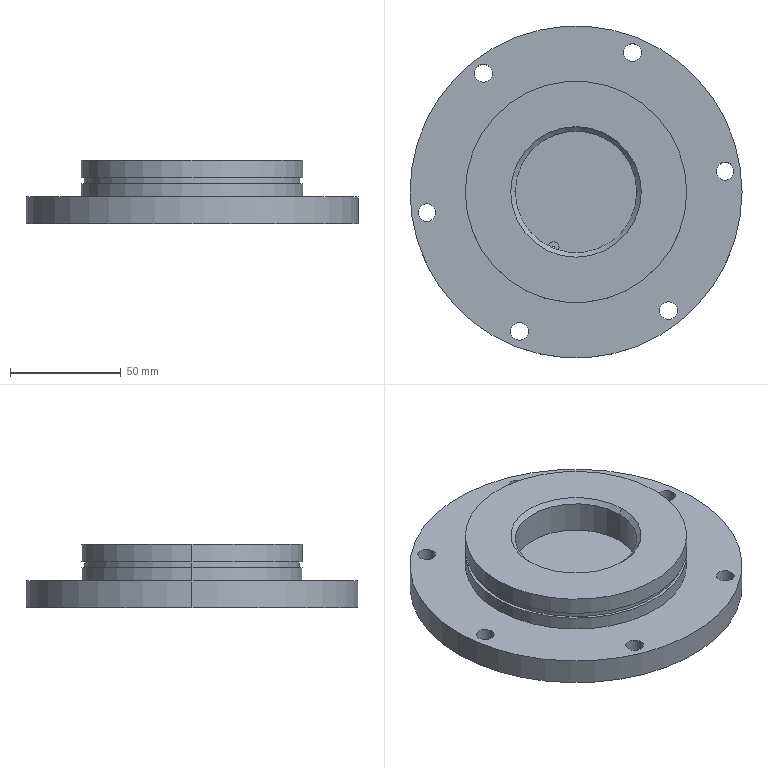Part | SolidWorks | features ICE 5, Chamfer 1, Extrusion 1 | 1 solid | 35 faces | box 150 x 150 x 28.5 mm | volume 297244 mm3 | cylinder 26 | plane 7 | cone 2 | commonest cylinder face diameters 8 x12 100 x4 1 x2 5 x2 55 x2 97.35 x2
STEP:
#1=CARTESIAN_POINT('',(-10.339,-25.483,12.));
#2=VERTEX_POINT('',#1);
#3=CARTESIAN_POINT('',(-9.651,-25.019,12.));
#4=VERTEX_POINT('',#3);
#5=CARTESIAN_POINT('',(-10.151,-25.019,12.));
#6=DIRECTION('',(0.,0.,1.));
#7=DIRECTION('',(1.,0.,0.));
#8=AXIS2_PLACEMENT_3D('',#5,#6,#7);
#9=CIRCLE('',#8,0.5);
#10=EDGE_CURVE('',#2,#4,#9,.T.);
#11=ORIENTED_EDGE('',*,*,#10,.T.);
#12=CARTESIAN_POINT('',(-9.651,-25.019,7.));
#13=VERTEX_POINT('',#12);
#14=CARTESIAN_POINT('',(-9.651,-25.019,28.5));
#15=DIRECTION('',(0.,0.,-1.));
#16=VECTOR('',#15,1000.);
#17=LINE('',#14,#16);
#18=EDGE_CURVE('',#4,#13,#17,.T.);
#19=ORIENTED_EDGE('',*,*,#18,.T.);
#20=CARTESIAN_POINT('',(-10.651,-25.019,7.));
#21=VERTEX_POINT('',#20);
#22=CARTESIAN_POINT('',(-10.151,-25.019,7.));
#23=DIRECTION('',(0.,0.,-1.));
#24=DIRECTION('',(-1.,0.,0.));
#25=AXIS2_PLACEMENT_3D('',#22,#23,#24);
#26=CIRCLE('',#25,0.5);
#27=EDGE_CURVE('',#13,#21,#26,.T.);
#28=ORIENTED_EDGE('',*,*,#27,.T.);
#29=CARTESIAN_POINT('',(-10.651,-25.019,12.));
#30=VERTEX_POINT('',#29);
#31=CARTESIAN_POINT('',(-10.651,-25.019,28.5));
#32=DIRECTION('',(0.,0.,-1.));
#33=VECTOR('',#32,1000.);
#34=LINE('',#31,#33);
#35=EDGE_CURVE('',#30,#21,#34,.T.);
#36=ORIENTED_EDGE('',*,*,#35,.F.);
#37=CARTESIAN_POINT('',(-10.151,-25.019,12.));
#38=DIRECTION('',(0.,0.,1.));
#39=DIRECTION('',(1.,0.,0.));
#40=AXIS2_PLACEMENT_3D('',#37,#38,#39);
#41=CIRCLE('',#40,0.5);
#42=EDGE_CURVE('',#30,#2,#41,.T.);
#43=ORIENTED_EDGE('',*,*,#42,.T.);
#44=EDGE_LOOP('',(#11,#19,#28,#36,#43));
#45=FACE_OUTER_BOUND('',#44,.T.);
#46=CARTESIAN_POINT('',(-10.151,-25.019,28.5));
#47=DIRECTION('',(0.,0.,-1.));
#48=DIRECTION('',(-1.,0.,0.));
#49=AXIS2_PLACEMENT_3D('',#46,#47,#48);
#50=CYLINDRICAL_SURFACE('',#49,0.5);
#51=ADVANCED_FACE('',(#45),#50,.F.);
#52=CARTESIAN_POINT('',(-7.651,-25.019,7.));
#53=VERTEX_POINT('',#52);
#54=CARTESIAN_POINT('',(-12.651,-25.019,7.));
#55=VERTEX_POINT('',#54);
#56=CARTESIAN_POINT('',(-10.151,-25.019,7.));
#57=DIRECTION('',(0.,0.,-1.));
#58=DIRECTION('',(-1.,0.,0.));
#59=AXIS2_PLACEMENT_3D('',#56,#57,#58);
#60=CIRCLE('',#59,2.5);
#61=EDGE_CURVE('',#53,#55,#60,.T.);
#62=ORIENTED_EDGE('',*,*,#61,.F.);
#63=CARTESIAN_POINT('',(-7.651,-25.019,0.));
#64=VERTEX_POINT('',#63);
#65=CARTESIAN_POINT('',(-7.651,-25.019,7.));
#66=DIRECTION('',(0.,0.,-1.));
#67=VECTOR('',#66,1000.);
#68=LINE('',#65,#67);
#69=EDGE_CURVE('',#53,#64,#68,.T.);
#70=ORIENTED_EDGE('',*,*,#69,.T.);
#71=CARTESIAN_POINT('',(-12.651,-25.019,0.));
#72=VERTEX_POINT('',#71);
#73=CARTESIAN_POINT('',(-10.151,-25.019,0.));
#74=DIRECTION('',(0.,0.,-1.));
#75=DIRECTION('',(-1.,0.,0.));
#76=AXIS2_PLACEMENT_3D('',#73,#74,#75);
#77=CIRCLE('',#76,2.5);
#78=EDGE_CURVE('',#64,#72,#77,.T.);
#79=ORIENTED_EDGE('',*,*,#78,.T.);
#80=CARTESIAN_POINT('',(-12.651,-25.019,7.));
#81=DIRECTION('',(0.,0.,-1.));
#82=VECTOR('',#81,1000.);
#83=LINE('',#80,#82);
#84=EDGE_CURVE('',#55,#72,#83,.T.);
#85=ORIENTED_EDGE('',*,*,#84,.F.);
#86=EDGE_LOOP('',(#62,#70,#79,#85));
#87=FACE_OUTER_BOUND('',#86,.T.);
#88=CARTESIAN_POINT('',(-10.151,-25.019,7.));
#89=DIRECTION('',(0.,0.,-1.));
#90=DIRECTION('',(-1.,0.,0.));
#91=AXIS2_PLACEMENT_3D('',#88,#89,#90);
#92=CYLINDRICAL_SURFACE('',#91,2.5);
#93=ADVANCED_FACE('',(#87),#92,.F.);
#94=CARTESIAN_POINT('',(21.565,63.011,12.));
#95=VERTEX_POINT('',#94);
#96=CARTESIAN_POINT('',(29.565,63.011,12.));
#97=VERTEX_POINT('',#96);
#98=CARTESIAN_POINT('',(25.565,63.011,12.));
#99=DIRECTION('',(0.,0.,1.));
#100=DIRECTION('',(1.,0.,0.));
#101=AXIS2_PLACEMENT_3D('',#98,#99,#100);
#102=CIRCLE('',#101,4.);
#103=EDGE_CURVE('',#95,#97,#102,.T.);
#104=ORIENTED_EDGE('',*,*,#103,.T.);
#105=CARTESIAN_POINT('',(29.565,63.011,0.));
#106=VERTEX_POINT('',#105);
#107=CARTESIAN_POINT('',(29.565,63.011,28.5));
#108=DIRECTION('',(0.,0.,-1.));
#109=VECTOR('',#108,1000.);
#110=LINE('',#107,#109);
#111=EDGE_CURVE('',#97,#106,#110,.T.);
#112=ORIENTED_EDGE('',*,*,#111,.T.);
#113=CARTESIAN_POINT('',(21.565,63.011,0.));
#114=VERTEX_POINT('',#113);
#115=CARTESIAN_POINT('',(25.565,63.011,0.));
#116=DIRECTION('',(0.,0.,-1.));
#117=DIRECTION('',(-1.,0.,0.));
#118=AXIS2_PLACEMENT_3D('',#115,#116,#117);
#119=CIRCLE('',#118,4.);
#120=EDGE_CURVE('',#106,#114,#119,.T.);
#121=ORIENTED_EDGE('',*,*,#120,.T.);
#122=CARTESIAN_POINT('',(21.565,63.011,28.5));
#123=DIRECTION('',(0.,0.,-1.));
#124=VECTOR('',#123,1000.);
#125=LINE('',#122,#124);
#126=EDGE_CURVE('',#95,#114,#125,.T.);
#127=ORIENTED_EDGE('',*,*,#126,.F.);
#128=EDGE_LOOP('',(#104,#112,#121,#127));
#129=FACE_OUTER_BOUND('',#128,.T.);
#130=CARTESIAN_POINT('',(25.565,63.011,28.5));
#131=DIRECTION('',(0.,0.,-1.));
#132=DIRECTION('',(-1.,0.,0.));
#133=AXIS2_PLACEMENT_3D('',#130,#131,#132);
#134=CYLINDRICAL_SURFACE('',#133,4.);
#135=ADVANCED_FACE('',(#129),#134,.F.);
#136=CARTESIAN_POINT('',(-45.787,53.645,12.));
#137=VERTEX_POINT('',#136);
#138=CARTESIAN_POINT('',(-37.787,53.645,12.));
#139=VERTEX_POINT('',#138);
#140=CARTESIAN_POINT('',(-41.787,53.645,12.));
#141=DIRECTION('',(0.,0.,1.));
#142=DIRECTION('',(1.,0.,0.));
#143=AXIS2_PLACEMENT_3D('',#140,#141,#142);
#144=CIRCLE('',#143,4.);
#145=EDGE_CURVE('',#137,#139,#144,.T.);
#146=ORIENTED_EDGE('',*,*,#145,.T.);
#147=CARTESIAN_POINT('',(-37.787,53.645,0.));
#148=VERTEX_POINT('',#147);
#149=CARTESIAN_POINT('',(-37.787,53.645,28.5));
#150=DIRECTION('',(0.,0.,-1.));
#151=VECTOR('',#150,1000.);
#152=LINE('',#149,#151);
#153=EDGE_CURVE('',#139,#148,#152,.T.);
#154=ORIENTED_EDGE('',*,*,#153,.T.);
#155=CARTESIAN_POINT('',(-45.787,53.645,0.));
#156=VERTEX_POINT('',#155);
#157=CARTESIAN_POINT('',(-41.787,53.645,0.));
#158=DIRECTION('',(0.,0.,-1.));
#159=DIRECTION('',(-1.,0.,0.));
#160=AXIS2_PLACEMENT_3D('',#157,#158,#159);
#161=CIRCLE('',#160,4.);
#162=EDGE_CURVE('',#148,#156,#161,.T.);
#163=ORIENTED_EDGE('',*,*,#162,.T.);
#164=CARTESIAN_POINT('',(-45.787,53.645,28.5));
#165=DIRECTION('',(0.,0.,-1.));
#166=VECTOR('',#165,1000.);
#167=LINE('',#164,#166);
#168=EDGE_CURVE('',#137,#156,#167,.T.);
#169=ORIENTED_EDGE('',*,*,#168,.F.);
#170=EDGE_LOOP('',(#146,#154,#163,#169));
#171=FACE_OUTER_BOUND('',#170,.T.);
#172=CARTESIAN_POINT('',(-41.787,53.645,28.5));
#173=DIRECTION('',(0.,0.,-1.));
#174=DIRECTION('',(-1.,0.,0.));
#175=AXIS2_PLACEMENT_3D('',#172,#173,#174);
#176=CYLINDRICAL_SURFACE('',#175,4.);
#177=ADVANCED_FACE('',(#171),#176,.F.);
#178=CARTESIAN_POINT('',(-71.352,-9.366,12.));
#179=VERTEX_POINT('',#178);
#180=CARTESIAN_POINT('',(-63.352,-9.366,12.));
#181=VERTEX_POINT('',#180);
#182=CARTESIAN_POINT('',(-67.352,-9.366,12.));
#183=DIRECTION('',(0.,0.,1.));
#184=DIRECTION('',(1.,0.,0.));
#185=AXIS2_PLACEMENT_3D('',#182,#183,#184);
#186=CIRCLE('',#185,4.);
#187=EDGE_CURVE('',#179,#181,#186,.T.);
#188=ORIENTED_EDGE('',*,*,#187,.T.);
#189=CARTESIAN_POINT('',(-63.352,-9.366,0.));
#190=VERTEX_POINT('',#189);
#191=CARTESIAN_POINT('',(-63.352,-9.366,28.5));
#192=DIRECTION('',(0.,0.,-1.));
#193=VECTOR('',#192,1000.);
#194=LINE('',#191,#193);
#195=EDGE_CURVE('',#181,#190,#194,.T.);
#196=ORIENTED_EDGE('',*,*,#195,.T.);
#197=CARTESIAN_POINT('',(-71.352,-9.366,0.));
#198=VERTEX_POINT('',#197);
#199=CARTESIAN_POINT('',(-67.352,-9.366,0.));
#200=DIRECTION('',(0.,0.,-1.));
#201=DIRECTION('',(-1.,0.,0.));
#202=AXIS2_PLACEMENT_3D('',#199,#200,#201);
#203=CIRCLE('',#202,4.);
#204=EDGE_CURVE('',#190,#198,#203,.T.);
#205=ORIENTED_EDGE('',*,*,#204,.T.);
#206=CARTESIAN_POINT('',(-71.352,-9.366,28.5));
#207=DIRECTION('',(0.,0.,-1.));
#208=VECTOR('',#207,1000.);
#209=LINE('',#206,#208);
#210=EDGE_CURVE('',#179,#198,#209,.T.);
#211=ORIENTED_EDGE('',*,*,#210,.F.);
#212=EDGE_LOOP('',(#188,#196,#205,#211));
#213=FACE_OUTER_BOUND('',#212,.T.);
#214=CARTESIAN_POINT('',(-67.352,-9.366,28.5));
#215=DIRECTION('',(0.,0.,-1.));
#216=DIRECTION('',(-1.,0.,0.));
#217=AXIS2_PLACEMENT_3D('',#214,#215,#216);
#218=CYLINDRICAL_SURFACE('',#217,4.);
#219=ADVANCED_FACE('',(#213),#218,.F.);
#220=CARTESIAN_POINT('',(-29.565,-63.011,12.));
#221=VERTEX_POINT('',#220);
#222=CARTESIAN_POINT('',(-21.565,-63.011,12.));
#223=VERTEX_POINT('',#222);
#224=CARTESIAN_POINT('',(-25.565,-63.011,12.));
#225=DIRECTION('',(0.,0.,1.));
#226=DIRECTION('',(1.,0.,0.));
#227=AXIS2_PLACEMENT_3D('',#224,#225,#226);
#228=CIRCLE('',#227,4.);
#229=EDGE_CURVE('',#221,#223,#228,.T.);
#230=ORIENTED_EDGE('',*,*,#229,.T.);
#231=CARTESIAN_POINT('',(-21.565,-63.011,0.));
#232=VERTEX_POINT('',#231);
#233=CARTESIAN_POINT('',(-21.565,-63.011,28.5));
#234=DIRECTION('',(0.,0.,-1.));
#235=VECTOR('',#234,1000.);
#236=LINE('',#233,#235);
#237=EDGE_CURVE('',#223,#232,#236,.T.);
#238=ORIENTED_EDGE('',*,*,#237,.T.);
#239=CARTESIAN_POINT('',(-29.565,-63.011,0.));
#240=VERTEX_POINT('',#239);
#241=CARTESIAN_POINT('',(-25.565,-63.011,0.));
#242=DIRECTION('',(0.,0.,-1.));
#243=DIRECTION('',(-1.,0.,0.));
#244=AXIS2_PLACEMENT_3D('',#241,#242,#243);
#245=CIRCLE('',#244,4.);
#246=EDGE_CURVE('',#232,#240,#245,.T.);
#247=ORIENTED_EDGE('',*,*,#246,.T.);
#248=CARTESIAN_POINT('',(-29.565,-63.011,28.5));
#249=DIRECTION('',(0.,0.,-1.));
#250=VECTOR('',#249,1000.);
#251=LINE('',#248,#250);
#252=EDGE_CURVE('',#221,#240,#251,.T.);
#253=ORIENTED_EDGE('',*,*,#252,.F.);
#254=EDGE_LOOP('',(#230,#238,#247,#253));
#255=FACE_OUTER_BOUND('',#254,.T.);
#256=CARTESIAN_POINT('',(-25.565,-63.011,28.5));
#257=DIRECTION('',(0.,0.,-1.));
#258=DIRECTION('',(-1.,0.,0.));
#259=AXIS2_PLACEMENT_3D('',#256,#257,#258);
#260=CYLINDRICAL_SURFACE('',#259,4.);
#261=ADVANCED_FACE('',(#255),#260,.F.);
#262=CARTESIAN_POINT('',(37.787,-53.645,12.));
#263=VERTEX_POINT('',#262);
#264=CARTESIAN_POINT('',(45.787,-53.645,12.));
#265=VERTEX_POINT('',#264);
#266=CARTESIAN_POINT('',(41.787,-53.645,12.));
#267=DIRECTION('',(0.,0.,1.));
#268=DIRECTION('',(1.,0.,0.));
#269=AXIS2_PLACEMENT_3D('',#266,#267,#268);
#270=CIRCLE('',#269,4.);
#271=EDGE_CURVE('',#263,#265,#270,.T.);
#272=ORIENTED_EDGE('',*,*,#271,.T.);
#273=CARTESIAN_POINT('',(45.787,-53.645,0.));
#274=VERTEX_POINT('',#273);
#275=CARTESIAN_POINT('',(45.787,-53.645,28.5));
#276=DIRECTION('',(0.,0.,-1.));
#277=VECTOR('',#276,1000.);
#278=LINE('',#275,#277);
#279=EDGE_CURVE('',#265,#274,#278,.T.);
#280=ORIENTED_EDGE('',*,*,#279,.T.);
#281=CARTESIAN_POINT('',(37.787,-53.645,0.));
#282=VERTEX_POINT('',#281);
#283=CARTESIAN_POINT('',(41.787,-53.645,0.));
#284=DIRECTION('',(0.,0.,-1.));
#285=DIRECTION('',(-1.,0.,0.));
#286=AXIS2_PLACEMENT_3D('',#283,#284,#285);
#287=CIRCLE('',#286,4.);
#288=EDGE_CURVE('',#274,#282,#287,.T.);
#289=ORIENTED_EDGE('',*,*,#288,.T.);
#290=CARTESIAN_POINT('',(37.787,-53.645,28.5));
#291=DIRECTION('',(0.,0.,-1.));
#292=VECTOR('',#291,1000.);
#293=LINE('',#290,#292);
#294=EDGE_CURVE('',#263,#282,#293,.T.);
#295=ORIENTED_EDGE('',*,*,#294,.F.);
#296=EDGE_LOOP('',(#272,#280,#289,#295));
#297=FACE_OUTER_BOUND('',#296,.T.);
#298=CARTESIAN_POINT('',(41.787,-53.645,28.5));
#299=DIRECTION('',(0.,0.,-1.));
#300=DIRECTION('',(-1.,0.,0.));
#301=AXIS2_PLACEMENT_3D('',#298,#299,#300);
#302=CYLINDRICAL_SURFACE('',#301,4.);
#303=ADVANCED_FACE('',(#297),#302,.F.);
#304=CARTESIAN_POINT('',(63.352,9.366,12.));
#305=VERTEX_POINT('',#304);
#306=CARTESIAN_POINT('',(71.352,9.366,12.));
#307=VERTEX_POINT('',#306);
#308=CARTESIAN_POINT('',(67.352,9.366,12.));
#309=DIRECTION('',(0.,0.,1.));
#310=DIRECTION('',(1.,0.,0.));
#311=AXIS2_PLACEMENT_3D('',#308,#309,#310);
#312=CIRCLE('',#311,4.);
#313=EDGE_CURVE('',#305,#307,#312,.T.);
#314=ORIENTED_EDGE('',*,*,#313,.T.);
#315=CARTESIAN_POINT('',(71.352,9.366,0.));
#316=VERTEX_POINT('',#315);
#317=CARTESIAN_POINT('',(71.352,9.366,28.5));
#318=DIRECTION('',(0.,0.,-1.));
#319=VECTOR('',#318,1000.);
#320=LINE('',#317,#319);
#321=EDGE_CURVE('',#307,#316,#320,.T.);
#322=ORIENTED_EDGE('',*,*,#321,.T.);
#323=CARTESIAN_POINT('',(63.352,9.366,0.));
#324=VERTEX_POINT('',#323);
#325=CARTESIAN_POINT('',(67.352,9.366,0.));
#326=DIRECTION('',(0.,0.,-1.));
#327=DIRECTION('',(-1.,0.,0.));
#328=AXIS2_PLACEMENT_3D('',#325,#326,#327);
#329=CIRCLE('',#328,4.);
#330=EDGE_CURVE('',#316,#324,#329,.T.);
#331=ORIENTED_EDGE('',*,*,#330,.T.);
#332=CARTESIAN_POINT('',(63.352,9.366,28.5));
#333=DIRECTION('',(0.,0.,-1.));
#334=VECTOR('',#333,1000.);
#335=LINE('',#332,#334);
#336=EDGE_CURVE('',#305,#324,#335,.T.);
#337=ORIENTED_EDGE('',*,*,#336,.F.);
#338=EDGE_LOOP('',(#314,#322,#331,#337));
#339=FACE_OUTER_BOUND('',#338,.T.);
#340=CARTESIAN_POINT('',(67.352,9.366,28.5));
#341=DIRECTION('',(0.,0.,-1.));
#342=DIRECTION('',(-1.,0.,0.));
#343=AXIS2_PLACEMENT_3D('',#340,#341,#342);
#344=CYLINDRICAL_SURFACE('',#343,4.);
#345=ADVANCED_FACE('',(#339),#344,.F.);
#346=CARTESIAN_POINT('',(-27.5,0.,26.5));
#347=VERTEX_POINT('',#346);
#348=CARTESIAN_POINT('',(27.5,0.,26.5));
#349=VERTEX_POINT('',#348);
#350=CARTESIAN_POINT('',(0.,0.,26.5));
#351=DIRECTION('',(0.,0.,1.));
#352=DIRECTION('',(1.,0.,0.));
#353=AXIS2_PLACEMENT_3D('',#350,#351,#352);
#354=CIRCLE('',#353,27.5);
#355=EDGE_CURVE('',#347,#349,#354,.T.);
#356=ORIENTED_EDGE('',*,*,#355,.F.);
#357=CARTESIAN_POINT('',(-29.5,0.,28.5));
#358=VERTEX_POINT('',#357);
#359=CARTESIAN_POINT('',(-27.5,0.,26.5));
#360=DIRECTION('',(-0.7071,0.,0.7071));
#361=VECTOR('',#360,1000.);
#362=LINE('',#359,#361);
#363=EDGE_CURVE('',#347,#358,#362,.T.);
#364=ORIENTED_EDGE('',*,*,#363,.T.);
#365=CARTESIAN_POINT('',(29.5,0.,28.5));
#366=VERTEX_POINT('',#365);
#367=CARTESIAN_POINT('',(0.,0.,28.5));
#368=DIRECTION('',(0.,0.,-1.));
#369=DIRECTION('',(1.,0.,0.));
#370=AXIS2_PLACEMENT_3D('',#367,#368,#369);
#371=CIRCLE('',#370,29.5);
#372=EDGE_CURVE('',#366,#358,#371,.T.);
#373=ORIENTED_EDGE('',*,*,#372,.F.);
#374=CARTESIAN_POINT('',(27.5,0.,26.5));
#375=DIRECTION('',(0.7071,0.,0.7071));
#376=VECTOR('',#375,1000.);
#377=LINE('',#374,#376);
#378=EDGE_CURVE('',#349,#366,#377,.T.);
#379=ORIENTED_EDGE('',*,*,#378,.F.);
#380=EDGE_LOOP('',(#356,#364,#373,#379));
#381=FACE_OUTER_BOUND('',#380,.T.);
#382=CARTESIAN_POINT('',(0.,0.,26.5));
#383=DIRECTION('',(0.,0.,1.));
#384=DIRECTION('',(1.,0.,0.));
#385=AXIS2_PLACEMENT_3D('',#382,#383,#384);
#386=CONICAL_SURFACE('',#385,27.5,0.7854);
#387=ADVANCED_FACE('',(#381),#386,.F.);
#388=CARTESIAN_POINT('',(-50.,0.,18.));
#389=VERTEX_POINT('',#388);
#390=CARTESIAN_POINT('',(50.,0.,18.));
#391=VERTEX_POINT('',#390);
#392=CARTESIAN_POINT('',(0.,0.,18.));
#393=DIRECTION('',(0.,0.,-1.));
#394=DIRECTION('',(-1.,0.,0.));
#395=AXIS2_PLACEMENT_3D('',#392,#393,#394);
#396=CIRCLE('',#395,50.);
#397=EDGE_CURVE('',#389,#391,#396,.T.);
#398=ORIENTED_EDGE('',*,*,#397,.T.);
#399=CARTESIAN_POINT('',(50.,0.,12.));
#400=VERTEX_POINT('',#399);
#401=CARTESIAN_POINT('',(50.,0.,28.5));
#402=DIRECTION('',(0.,0.,-1.));
#403=VECTOR('',#402,1000.);
#404=LINE('',#401,#403);
#405=EDGE_CURVE('',#391,#400,#404,.T.);
#406=ORIENTED_EDGE('',*,*,#405,.T.);
#407=CARTESIAN_POINT('',(-50.,0.,12.));
#408=VERTEX_POINT('',#407);
#409=CARTESIAN_POINT('',(0.,0.,12.));
#410=DIRECTION('',(0.,0.,-1.));
#411=DIRECTION('',(1.,0.,0.));
#412=AXIS2_PLACEMENT_3D('',#409,#410,#411);
#413=CIRCLE('',#412,50.);
#414=EDGE_CURVE('',#408,#400,#413,.T.);
#415=ORIENTED_EDGE('',*,*,#414,.F.);
#416=CARTESIAN_POINT('',(-50.,0.,28.5));
#417=DIRECTION('',(0.,0.,-1.));
#418=VECTOR('',#417,1000.);
#419=LINE('',#416,#418);
#420=EDGE_CURVE('',#389,#408,#419,.T.);
#421=ORIENTED_EDGE('',*,*,#420,.F.);
#422=EDGE_LOOP('',(#398,#406,#415,#421));
#423=FACE_OUTER_BOUND('',#422,.T.);
#424=CARTESIAN_POINT('',(0.,0.,28.5));
#425=DIRECTION('',(0.,0.,-1.));
#426=DIRECTION('',(-1.,0.,0.));
#427=AXIS2_PLACEMENT_3D('',#424,#425,#426);
#428=CYLINDRICAL_SURFACE('',#427,50.);
#429=ADVANCED_FACE('',(#423),#428,.T.);
#430=CARTESIAN_POINT('',(75.,0.,12.));
#431=VERTEX_POINT('',#430);
#432=CARTESIAN_POINT('',(-75.,0.,12.));
#433=VERTEX_POINT('',#432);
#434=CARTESIAN_POINT('',(0.,0.,12.));
#435=DIRECTION('',(0.,0.,1.));
#436=DIRECTION('',(1.,0.,0.));
#437=AXIS2_PLACEMENT_3D('',#434,#435,#436);
#438=CIRCLE('',#437,75.);
#439=EDGE_CURVE('',#431,#433,#438,.T.);
#440=ORIENTED_EDGE('',*,*,#439,.F.);
#441=CARTESIAN_POINT('',(75.,0.,0.));
#442=VERTEX_POINT('',#441);
#443=CARTESIAN_POINT('',(75.,0.,12.));
#444=DIRECTION('',(0.,0.,-1.));
#445=VECTOR('',#444,1000.);
#446=LINE('',#443,#445);
#447=EDGE_CURVE('',#431,#442,#446,.T.);
#448=ORIENTED_EDGE('',*,*,#447,.T.);
#449=CARTESIAN_POINT('',(-75.,0.,0.));
#450=VERTEX_POINT('',#449);
#451=CARTESIAN_POINT('',(0.,0.,0.));
#452=DIRECTION('',(0.,0.,1.));
#453=DIRECTION('',(1.,0.,0.));
#454=AXIS2_PLACEMENT_3D('',#451,#452,#453);
#455=CIRCLE('',#454,75.);
#456=EDGE_CURVE('',#442,#450,#455,.T.);
#457=ORIENTED_EDGE('',*,*,#456,.T.);
#458=CARTESIAN_POINT('',(-75.,0.,12.));
#459=DIRECTION('',(0.,0.,-1.));
#460=VECTOR('',#459,1000.);
#461=LINE('',#458,#460);
#462=EDGE_CURVE('',#433,#450,#461,.T.);
#463=ORIENTED_EDGE('',*,*,#462,.F.);
#464=EDGE_LOOP('',(#440,#448,#457,#463));
#465=FACE_OUTER_BOUND('',#464,.T.);
#466=CARTESIAN_POINT('',(0.,0.,12.));
#467=DIRECTION('',(0.,0.,-1.));
#468=DIRECTION('',(-1.,0.,0.));
#469=AXIS2_PLACEMENT_3D('',#466,#467,#468);
#470=CYLINDRICAL_SURFACE('',#469,75.);
#471=ADVANCED_FACE('',(#465),#470,.T.);
#472=CARTESIAN_POINT('',(-48.675,0.,20.65));
#473=VERTEX_POINT('',#472);
#474=CARTESIAN_POINT('',(48.675,0.,20.65));
#475=VERTEX_POINT('',#474);
#476=CARTESIAN_POINT('',(0.,0.,20.65));
#477=DIRECTION('',(0.,0.,-1.));
#478=DIRECTION('',(-1.,0.,0.));
#479=AXIS2_PLACEMENT_3D('',#476,#477,#478);
#480=CIRCLE('',#479,48.675);
#481=EDGE_CURVE('',#473,#475,#480,.T.);
#482=ORIENTED_EDGE('',*,*,#481,.T.);
#483=CARTESIAN_POINT('',(48.675,0.,18.));
#484=VERTEX_POINT('',#483);
#485=CARTESIAN_POINT('',(48.675,0.,20.65));
#486=DIRECTION('',(0.,0.,-1.));
#487=VECTOR('',#486,1000.);
#488=LINE('',#485,#487);
#489=EDGE_CURVE('',#475,#484,#488,.T.);
#490=ORIENTED_EDGE('',*,*,#489,.T.);
#491=CARTESIAN_POINT('',(-48.675,0.,18.));
#492=VERTEX_POINT('',#491);
#493=CARTESIAN_POINT('',(0.,0.,18.));
#494=DIRECTION('',(0.,0.,-1.));
#495=DIRECTION('',(-1.,0.,0.));
#496=AXIS2_PLACEMENT_3D('',#493,#494,#495);
#497=CIRCLE('',#496,48.675);
#498=EDGE_CURVE('',#492,#484,#497,.T.);
#499=ORIENTED_EDGE('',*,*,#498,.F.);
#500=CARTESIAN_POINT('',(-48.675,0.,20.65));
#501=DIRECTION('',(0.,0.,-1.));
#502=VECTOR('',#501,1000.);
#503=LINE('',#500,#502);
#504=EDGE_CURVE('',#473,#492,#503,.T.);
#505=ORIENTED_EDGE('',*,*,#504,.F.);
#506=EDGE_LOOP('',(#482,#490,#499,#505));
#507=FACE_OUTER_BOUND('',#506,.T.);
#508=CARTESIAN_POINT('',(0.,0.,20.65));
#509=DIRECTION('',(0.,0.,-1.));
#510=DIRECTION('',(-1.,0.,0.));
#511=AXIS2_PLACEMENT_3D('',#508,#509,#510);
#512=CYLINDRICAL_SURFACE('',#511,48.675);
#513=ADVANCED_FACE('',(#507),#512,.T.);
#514=ORIENTED_EDGE('',*,*,#355,.T.);
#515=CARTESIAN_POINT('',(27.5,0.,12.));
#516=VERTEX_POINT('',#515);
#517=CARTESIAN_POINT('',(27.5,0.,28.5));
#518=DIRECTION('',(0.,0.,-1.));
#519=VECTOR('',#518,1000.);
#520=LINE('',#517,#519);
#521=EDGE_CURVE('',#349,#516,#520,.T.);
#522=ORIENTED_EDGE('',*,*,#521,.T.);
#523=CARTESIAN_POINT('',(0.,0.,12.));
#524=DIRECTION('',(0.,0.,-1.));
#525=DIRECTION('',(1.,0.,0.));
#526=AXIS2_PLACEMENT_3D('',#523,#524,#525);
#527=CIRCLE('',#526,27.5);
#528=EDGE_CURVE('',#516,#2,#527,.T.);
#529=ORIENTED_EDGE('',*,*,#528,.T.);
#530=CARTESIAN_POINT('',(-27.5,0.,12.));
#531=VERTEX_POINT('',#530);
#532=CARTESIAN_POINT('',(0.,0.,12.));
#533=DIRECTION('',(0.,0.,-1.));
#534=DIRECTION('',(1.,0.,0.));
#535=AXIS2_PLACEMENT_3D('',#532,#533,#534);
#536=CIRCLE('',#535,27.5);
#537=EDGE_CURVE('',#2,#531,#536,.T.);
#538=ORIENTED_EDGE('',*,*,#537,.T.);
#539=CARTESIAN_POINT('',(-27.5,0.,28.5));
#540=DIRECTION('',(0.,0.,-1.));
#541=VECTOR('',#540,1000.);
#542=LINE('',#539,#541);
#543=EDGE_CURVE('',#347,#531,#542,.T.);
#544=ORIENTED_EDGE('',*,*,#543,.F.);
#545=EDGE_LOOP('',(#514,#522,#529,#538,#544));
#546=FACE_OUTER_BOUND('',#545,.T.);
#547=CARTESIAN_POINT('',(0.,0.,28.5));
#548=DIRECTION('',(0.,0.,-1.));
#549=DIRECTION('',(-1.,0.,0.));
#550=AXIS2_PLACEMENT_3D('',#547,#548,#549);
#551=CYLINDRICAL_SURFACE('',#550,27.5);
#552=ADVANCED_FACE('',(#546),#551,.F.);
#553=CARTESIAN_POINT('',(50.,0.,28.5));
#554=VERTEX_POINT('',#553);
#555=CARTESIAN_POINT('',(-50.,0.,28.5));
#556=VERTEX_POINT('',#555);
#557=CARTESIAN_POINT('',(0.,0.,28.5));
#558=DIRECTION('',(0.,0.,1.));
#559=DIRECTION('',(1.,0.,0.));
#560=AXIS2_PLACEMENT_3D('',#557,#558,#559);
#561=CIRCLE('',#560,50.);
#562=EDGE_CURVE('',#554,#556,#561,.T.);
#563=ORIENTED_EDGE('',*,*,#562,.F.);
#564=CARTESIAN_POINT('',(50.,0.,20.65));
#565=VERTEX_POINT('',#564);
#566=CARTESIAN_POINT('',(50.,0.,28.5));
#567=DIRECTION('',(0.,0.,-1.));
#568=VECTOR('',#567,1000.);
#569=LINE('',#566,#568);
#570=EDGE_CURVE('',#554,#565,#569,.T.);
#571=ORIENTED_EDGE('',*,*,#570,.T.);
#572=CARTESIAN_POINT('',(-50.,0.,20.65));
#573=VERTEX_POINT('',#572);
#574=CARTESIAN_POINT('',(0.,0.,20.65));
#575=DIRECTION('',(0.,0.,-1.));
#576=DIRECTION('',(-1.,0.,0.));
#577=AXIS2_PLACEMENT_3D('',#574,#575,#576);
#578=CIRCLE('',#577,50.);
#579=EDGE_CURVE('',#573,#565,#578,.T.);
#580=ORIENTED_EDGE('',*,*,#579,.F.);
#581=CARTESIAN_POINT('',(-50.,0.,28.5));
#582=DIRECTION('',(0.,0.,-1.));
#583=VECTOR('',#582,1000.);
#584=LINE('',#581,#583);
#585=EDGE_CURVE('',#556,#573,#584,.T.);
#586=ORIENTED_EDGE('',*,*,#585,.F.);
#587=EDGE_LOOP('',(#563,#571,#580,#586));
#588=FACE_OUTER_BOUND('',#587,.T.);
#589=CARTESIAN_POINT('',(0.,0.,28.5));
#590=DIRECTION('',(0.,0.,-1.));
#591=DIRECTION('',(-1.,0.,0.));
#592=AXIS2_PLACEMENT_3D('',#589,#590,#591);
#593=CYLINDRICAL_SURFACE('',#592,50.);
#594=ADVANCED_FACE('',(#588),#593,.T.);
#595=ORIENTED_EDGE('',*,*,#570,.F.);
#596=CARTESIAN_POINT('',(0.,0.,28.5));
#597=DIRECTION('',(0.,0.,1.));
#598=DIRECTION('',(1.,0.,0.));
#599=AXIS2_PLACEMENT_3D('',#596,#597,#598);
#600=CIRCLE('',#599,50.);
#601=EDGE_CURVE('',#556,#554,#600,.T.);
#602=ORIENTED_EDGE('',*,*,#601,.F.);
#603=ORIENTED_EDGE('',*,*,#585,.T.);
#604=CARTESIAN_POINT('',(0.,0.,20.65));
#605=DIRECTION('',(0.,0.,-1.));
#606=DIRECTION('',(-1.,0.,0.));
#607=AXIS2_PLACEMENT_3D('',#604,#605,#606);
#608=CIRCLE('',#607,50.);
#609=EDGE_CURVE('',#565,#573,#608,.T.);
#610=ORIENTED_EDGE('',*,*,#609,.F.);
#611=EDGE_LOOP('',(#595,#602,#603,#610));
#612=FACE_OUTER_BOUND('',#611,.T.);
#613=CARTESIAN_POINT('',(0.,0.,28.5));
#614=DIRECTION('',(0.,0.,-1.));
#615=DIRECTION('',(-1.,0.,0.));
#616=AXIS2_PLACEMENT_3D('',#613,#614,#615);
#617=CYLINDRICAL_SURFACE('',#616,50.);
#618=ADVANCED_FACE('',(#612),#617,.T.);
#619=ORIENTED_EDGE('',*,*,#372,.T.);
#620=CARTESIAN_POINT('',(0.,0.,28.5));
#621=DIRECTION('',(0.,0.,-1.));
#622=DIRECTION('',(1.,0.,0.));
#623=AXIS2_PLACEMENT_3D('',#620,#621,#622);
#624=CIRCLE('',#623,29.5);
#625=EDGE_CURVE('',#358,#366,#624,.T.);
#626=ORIENTED_EDGE('',*,*,#625,.T.);
#627=EDGE_LOOP('',(#619,#626));
#628=FACE_BOUND('',#627,.T.);
#629=ORIENTED_EDGE('',*,*,#601,.T.);
#630=ORIENTED_EDGE('',*,*,#562,.T.);
#631=EDGE_LOOP('',(#629,#630));
#632=FACE_OUTER_BOUND('',#631,.T.);
#633=CARTESIAN_POINT('',(0.,0.,28.5));
#634=DIRECTION('',(0.,0.,1.));
#635=DIRECTION('',(1.,0.,0.));
#636=AXIS2_PLACEMENT_3D('',#633,#634,#635);
#637=PLANE('',#636);
#638=ADVANCED_FACE('',(#628,#632),#637,.T.);
#639=ORIENTED_EDGE('',*,*,#521,.F.);
#640=CARTESIAN_POINT('',(0.,0.,26.5));
#641=DIRECTION('',(0.,0.,1.));
#642=DIRECTION('',(1.,0.,0.));
#643=AXIS2_PLACEMENT_3D('',#640,#641,#642);
#644=CIRCLE('',#643,27.5);
#645=EDGE_CURVE('',#349,#347,#644,.T.);
#646=ORIENTED_EDGE('',*,*,#645,.T.);
#647=ORIENTED_EDGE('',*,*,#543,.T.);
#648=CARTESIAN_POINT('',(0.,0.,12.));
#649=DIRECTION('',(0.,0.,-1.));
#650=DIRECTION('',(1.,0.,0.));
#651=AXIS2_PLACEMENT_3D('',#648,#649,#650);
#652=CIRCLE('',#651,27.5);
#653=EDGE_CURVE('',#531,#516,#652,.T.);
#654=ORIENTED_EDGE('',*,*,#653,.T.);
#655=EDGE_LOOP('',(#639,#646,#647,#654));
#656=FACE_OUTER_BOUND('',#655,.T.);
#657=CARTESIAN_POINT('',(0.,0.,28.5));
#658=DIRECTION('',(0.,0.,-1.));
#659=DIRECTION('',(-1.,0.,0.));
#660=AXIS2_PLACEMENT_3D('',#657,#658,#659);
#661=CYLINDRICAL_SURFACE('',#660,27.5);
#662=ADVANCED_FACE('',(#656),#661,.F.);
#663=ORIENTED_EDGE('',*,*,#537,.F.);
#664=ORIENTED_EDGE('',*,*,#42,.F.);
#665=CARTESIAN_POINT('',(-10.151,-25.019,12.));
#666=DIRECTION('',(0.,0.,1.));
#667=DIRECTION('',(1.,0.,0.));
#668=AXIS2_PLACEMENT_3D('',#665,#666,#667);
#669=CIRCLE('',#668,0.5);
#670=EDGE_CURVE('',#4,#30,#669,.T.);
#671=ORIENTED_EDGE('',*,*,#670,.F.);
#672=ORIENTED_EDGE('',*,*,#10,.F.);
#673=ORIENTED_EDGE('',*,*,#528,.F.);
#674=ORIENTED_EDGE('',*,*,#653,.F.);
#675=EDGE_LOOP('',(#663,#664,#671,#672,#673,#674));
#676=FACE_OUTER_BOUND('',#675,.T.);
#677=CARTESIAN_POINT('',(0.,0.,12.));
#678=DIRECTION('',(0.,0.,1.));
#679=DIRECTION('',(1.,0.,0.));
#680=AXIS2_PLACEMENT_3D('',#677,#678,#679);
#681=PLANE('',#680);
#682=ADVANCED_FACE('',(#676),#681,.T.);
#683=ORIENTED_EDGE('',*,*,#481,.F.);
#684=CARTESIAN_POINT('',(0.,0.,20.65));
#685=DIRECTION('',(0.,0.,-1.));
#686=DIRECTION('',(-1.,0.,0.));
#687=AXIS2_PLACEMENT_3D('',#684,#685,#686);
#688=CIRCLE('',#687,48.675);
#689=EDGE_CURVE('',#475,#473,#688,.T.);
#690=ORIENTED_EDGE('',*,*,#689,.F.);
#691=EDGE_LOOP('',(#683,#690));
#692=FACE_BOUND('',#691,.T.);
#693=ORIENTED_EDGE('',*,*,#579,.T.);
#694=ORIENTED_EDGE('',*,*,#609,.T.);
#695=EDGE_LOOP('',(#693,#694));
#696=FACE_OUTER_BOUND('',#695,.T.);
#697=CARTESIAN_POINT('',(0.,0.,20.65));
#698=DIRECTION('',(0.,0.,-1.));
#699=DIRECTION('',(-1.,0.,0.));
#700=AXIS2_PLACEMENT_3D('',#697,#698,#699);
#701=PLANE('',#700);
#702=ADVANCED_FACE('',(#692,#696),#701,.T.);
#703=ORIENTED_EDGE('',*,*,#498,.T.);
#704=CARTESIAN_POINT('',(0.,0.,18.));
#705=DIRECTION('',(0.,0.,-1.));
#706=DIRECTION('',(-1.,0.,0.));
#707=AXIS2_PLACEMENT_3D('',#704,#705,#706);
#708=CIRCLE('',#707,48.675);
#709=EDGE_CURVE('',#484,#492,#708,.T.);
#710=ORIENTED_EDGE('',*,*,#709,.T.);
#711=EDGE_LOOP('',(#703,#710));
#712=FACE_BOUND('',#711,.T.);
#713=ORIENTED_EDGE('',*,*,#397,.F.);
#714=CARTESIAN_POINT('',(0.,0.,18.));
#715=DIRECTION('',(0.,0.,-1.));
#716=DIRECTION('',(-1.,0.,0.));
#717=AXIS2_PLACEMENT_3D('',#714,#715,#716);
#718=CIRCLE('',#717,50.);
#719=EDGE_CURVE('',#391,#389,#718,.T.);
#720=ORIENTED_EDGE('',*,*,#719,.F.);
#721=EDGE_LOOP('',(#713,#720));
#722=FACE_OUTER_BOUND('',#721,.T.);
#723=CARTESIAN_POINT('',(0.,0.,18.));
#724=DIRECTION('',(0.,0.,-1.));
#725=DIRECTION('',(-1.,0.,0.));
#726=AXIS2_PLACEMENT_3D('',#723,#724,#725);
#727=PLANE('',#726);
#728=ADVANCED_FACE('',(#712,#722),#727,.F.);
#729=ORIENTED_EDGE('',*,*,#489,.F.);
#730=ORIENTED_EDGE('',*,*,#689,.T.);
#731=ORIENTED_EDGE('',*,*,#504,.T.);
#732=ORIENTED_EDGE('',*,*,#709,.F.);
#733=EDGE_LOOP('',(#729,#730,#731,#732));
#734=FACE_OUTER_BOUND('',#733,.T.);
#735=CARTESIAN_POINT('',(0.,0.,20.65));
#736=DIRECTION('',(0.,0.,-1.));
#737=DIRECTION('',(-1.,0.,0.));
#738=AXIS2_PLACEMENT_3D('',#735,#736,#737);
#739=CYLINDRICAL_SURFACE('',#738,48.675);
#740=ADVANCED_FACE('',(#734),#739,.T.);
#741=CARTESIAN_POINT('',(-10.151,-25.019,0.));
#742=DIRECTION('',(0.,0.,-1.));
#743=DIRECTION('',(-1.,0.,0.));
#744=AXIS2_PLACEMENT_3D('',#741,#742,#743);
#745=CIRCLE('',#744,2.5);
#746=EDGE_CURVE('',#72,#64,#745,.T.);
#747=ORIENTED_EDGE('',*,*,#746,.F.);
#748=ORIENTED_EDGE('',*,*,#78,.F.);
#749=EDGE_LOOP('',(#747,#748));
#750=FACE_BOUND('',#749,.T.);
#751=CARTESIAN_POINT('',(25.565,63.011,0.));
#752=DIRECTION('',(0.,0.,-1.));
#753=DIRECTION('',(-1.,0.,0.));
#754=AXIS2_PLACEMENT_3D('',#751,#752,#753);
#755=CIRCLE('',#754,4.);
#756=EDGE_CURVE('',#114,#106,#755,.T.);
#757=ORIENTED_EDGE('',*,*,#756,.F.);
#758=ORIENTED_EDGE('',*,*,#120,.F.);
#759=EDGE_LOOP('',(#757,#758));
#760=FACE_BOUND('',#759,.T.);
#761=CARTESIAN_POINT('',(-41.787,53.645,0.));
#762=DIRECTION('',(0.,0.,-1.));
#763=DIRECTION('',(-1.,0.,0.));
#764=AXIS2_PLACEMENT_3D('',#761,#762,#763);
#765=CIRCLE('',#764,4.);
#766=EDGE_CURVE('',#156,#148,#765,.T.);
#767=ORIENTED_EDGE('',*,*,#766,.F.);
#768=ORIENTED_EDGE('',*,*,#162,.F.);
#769=EDGE_LOOP('',(#767,#768));
#770=FACE_BOUND('',#769,.T.);
#771=CARTESIAN_POINT('',(-67.352,-9.366,0.));
#772=DIRECTION('',(0.,0.,-1.));
#773=DIRECTION('',(-1.,0.,0.));
#774=AXIS2_PLACEMENT_3D('',#771,#772,#773);
#775=CIRCLE('',#774,4.);
#776=EDGE_CURVE('',#198,#190,#775,.T.);
#777=ORIENTED_EDGE('',*,*,#776,.F.);
#778=ORIENTED_EDGE('',*,*,#204,.F.);
#779=EDGE_LOOP('',(#777,#778));
#780=FACE_BOUND('',#779,.T.);
#781=CARTESIAN_POINT('',(-25.565,-63.011,0.));
#782=DIRECTION('',(0.,0.,-1.));
#783=DIRECTION('',(-1.,0.,0.));
#784=AXIS2_PLACEMENT_3D('',#781,#782,#783);
#785=CIRCLE('',#784,4.);
#786=EDGE_CURVE('',#240,#232,#785,.T.);
#787=ORIENTED_EDGE('',*,*,#786,.F.);
#788=ORIENTED_EDGE('',*,*,#246,.F.);
#789=EDGE_LOOP('',(#787,#788));
#790=FACE_BOUND('',#789,.T.);
#791=CARTESIAN_POINT('',(41.787,-53.645,0.));
#792=DIRECTION('',(0.,0.,-1.));
#793=DIRECTION('',(-1.,0.,0.));
#794=AXIS2_PLACEMENT_3D('',#791,#792,#793);
#795=CIRCLE('',#794,4.);
#796=EDGE_CURVE('',#282,#274,#795,.T.);
#797=ORIENTED_EDGE('',*,*,#796,.F.);
#798=ORIENTED_EDGE('',*,*,#288,.F.);
#799=EDGE_LOOP('',(#797,#798));
#800=FACE_BOUND('',#799,.T.);
#801=CARTESIAN_POINT('',(67.352,9.366,0.));
#802=DIRECTION('',(0.,0.,-1.));
#803=DIRECTION('',(-1.,0.,0.));
#804=AXIS2_PLACEMENT_3D('',#801,#802,#803);
#805=CIRCLE('',#804,4.);
#806=EDGE_CURVE('',#324,#316,#805,.T.);
#807=ORIENTED_EDGE('',*,*,#806,.F.);
#808=ORIENTED_EDGE('',*,*,#330,.F.);
#809=EDGE_LOOP('',(#807,#808));
#810=FACE_BOUND('',#809,.T.);
#811=CARTESIAN_POINT('',(0.,0.,0.));
#812=DIRECTION('',(0.,0.,1.));
#813=DIRECTION('',(1.,0.,0.));
#814=AXIS2_PLACEMENT_3D('',#811,#812,#813);
#815=CIRCLE('',#814,75.);
#816=EDGE_CURVE('',#450,#442,#815,.T.);
#817=ORIENTED_EDGE('',*,*,#816,.F.);
#818=ORIENTED_EDGE('',*,*,#456,.F.);
#819=EDGE_LOOP('',(#817,#818));
#820=FACE_OUTER_BOUND('',#819,.T.);
#821=CARTESIAN_POINT('',(0.,0.,0.));
#822=DIRECTION('',(0.,0.,1.));
#823=DIRECTION('',(1.,0.,0.));
#824=AXIS2_PLACEMENT_3D('',#821,#822,#823);
#825=PLANE('',#824);
#826=ADVANCED_FACE('',(#750,#760,#770,#780,#790,#800,#810,#820),#825,.F.);
#827=ORIENTED_EDGE('',*,*,#447,.F.);
#828=CARTESIAN_POINT('',(0.,0.,12.));
#829=DIRECTION('',(0.,0.,1.));
#830=DIRECTION('',(1.,0.,0.));
#831=AXIS2_PLACEMENT_3D('',#828,#829,#830);
#832=CIRCLE('',#831,75.);
#833=EDGE_CURVE('',#433,#431,#832,.T.);
#834=ORIENTED_EDGE('',*,*,#833,.F.);
#835=ORIENTED_EDGE('',*,*,#462,.T.);
#836=ORIENTED_EDGE('',*,*,#816,.T.);
#837=EDGE_LOOP('',(#827,#834,#835,#836));
#838=FACE_OUTER_BOUND('',#837,.T.);
#839=CARTESIAN_POINT('',(0.,0.,12.));
#840=DIRECTION('',(0.,0.,-1.));
#841=DIRECTION('',(-1.,0.,0.));
#842=AXIS2_PLACEMENT_3D('',#839,#840,#841);
#843=CYLINDRICAL_SURFACE('',#842,75.);
#844=ADVANCED_FACE('',(#838),#843,.T.);
#845=ORIENTED_EDGE('',*,*,#103,.F.);
#846=CARTESIAN_POINT('',(25.565,63.011,12.));
#847=DIRECTION('',(0.,0.,1.));
#848=DIRECTION('',(1.,0.,0.));
#849=AXIS2_PLACEMENT_3D('',#846,#847,#848);
#850=CIRCLE('',#849,4.);
#851=EDGE_CURVE('',#97,#95,#850,.T.);
#852=ORIENTED_EDGE('',*,*,#851,.F.);
#853=EDGE_LOOP('',(#845,#852));
#854=FACE_BOUND('',#853,.T.);
#855=ORIENTED_EDGE('',*,*,#145,.F.);
#856=CARTESIAN_POINT('',(-41.787,53.645,12.));
#857=DIRECTION('',(0.,0.,1.));
#858=DIRECTION('',(1.,0.,0.));
#859=AXIS2_PLACEMENT_3D('',#856,#857,#858);
#860=CIRCLE('',#859,4.);
#861=EDGE_CURVE('',#139,#137,#860,.T.);
#862=ORIENTED_EDGE('',*,*,#861,.F.);
#863=EDGE_LOOP('',(#855,#862));
#864=FACE_BOUND('',#863,.T.);
#865=ORIENTED_EDGE('',*,*,#187,.F.);
#866=CARTESIAN_POINT('',(-67.352,-9.366,12.));
#867=DIRECTION('',(0.,0.,1.));
#868=DIRECTION('',(1.,0.,0.));
#869=AXIS2_PLACEMENT_3D('',#866,#867,#868);
#870=CIRCLE('',#869,4.);
#871=EDGE_CURVE('',#181,#179,#870,.T.);
#872=ORIENTED_EDGE('',*,*,#871,.F.);
#873=EDGE_LOOP('',(#865,#872));
#874=FACE_BOUND('',#873,.T.);
#875=ORIENTED_EDGE('',*,*,#229,.F.);
#876=CARTESIAN_POINT('',(-25.565,-63.011,12.));
#877=DIRECTION('',(0.,0.,1.));
#878=DIRECTION('',(1.,0.,0.));
#879=AXIS2_PLACEMENT_3D('',#876,#877,#878);
#880=CIRCLE('',#879,4.);
#881=EDGE_CURVE('',#223,#221,#880,.T.);
#882=ORIENTED_EDGE('',*,*,#881,.F.);
#883=EDGE_LOOP('',(#875,#882));
#884=FACE_BOUND('',#883,.T.);
#885=ORIENTED_EDGE('',*,*,#271,.F.);
#886=CARTESIAN_POINT('',(41.787,-53.645,12.));
#887=DIRECTION('',(0.,0.,1.));
#888=DIRECTION('',(1.,0.,0.));
#889=AXIS2_PLACEMENT_3D('',#886,#887,#888);
#890=CIRCLE('',#889,4.);
#891=EDGE_CURVE('',#265,#263,#890,.T.);
#892=ORIENTED_EDGE('',*,*,#891,.F.);
#893=EDGE_LOOP('',(#885,#892));
#894=FACE_BOUND('',#893,.T.);
#895=ORIENTED_EDGE('',*,*,#313,.F.);
#896=CARTESIAN_POINT('',(67.352,9.366,12.));
#897=DIRECTION('',(0.,0.,1.));
#898=DIRECTION('',(1.,0.,0.));
#899=AXIS2_PLACEMENT_3D('',#896,#897,#898);
#900=CIRCLE('',#899,4.);
#901=EDGE_CURVE('',#307,#305,#900,.T.);
#902=ORIENTED_EDGE('',*,*,#901,.F.);
#903=EDGE_LOOP('',(#895,#902));
#904=FACE_BOUND('',#903,.T.);
#905=ORIENTED_EDGE('',*,*,#414,.T.);
#906=CARTESIAN_POINT('',(0.,0.,12.));
#907=DIRECTION('',(0.,0.,-1.));
#908=DIRECTION('',(1.,0.,0.));
#909=AXIS2_PLACEMENT_3D('',#906,#907,#908);
#910=CIRCLE('',#909,50.);
#911=EDGE_CURVE('',#400,#408,#910,.T.);
#912=ORIENTED_EDGE('',*,*,#911,.T.);
#913=EDGE_LOOP('',(#905,#912));
#914=FACE_BOUND('',#913,.T.);
#915=ORIENTED_EDGE('',*,*,#833,.T.);
#916=ORIENTED_EDGE('',*,*,#439,.T.);
#917=EDGE_LOOP('',(#915,#916));
#918=FACE_OUTER_BOUND('',#917,.T.);
#919=CARTESIAN_POINT('',(0.,0.,12.));
#920=DIRECTION('',(0.,0.,1.));
#921=DIRECTION('',(1.,0.,0.));
#922=AXIS2_PLACEMENT_3D('',#919,#920,#921);
#923=PLANE('',#922);
#924=ADVANCED_FACE('',(#854,#864,#874,#884,#894,#904,#914,#918),#923,.T.);
#925=ORIENTED_EDGE('',*,*,#405,.F.);
#926=ORIENTED_EDGE('',*,*,#719,.T.);
#927=ORIENTED_EDGE('',*,*,#420,.T.);
#928=ORIENTED_EDGE('',*,*,#911,.F.);
#929=EDGE_LOOP('',(#925,#926,#927,#928));
#930=FACE_OUTER_BOUND('',#929,.T.);
#931=CARTESIAN_POINT('',(0.,0.,28.5));
#932=DIRECTION('',(0.,0.,-1.));
#933=DIRECTION('',(-1.,0.,0.));
#934=AXIS2_PLACEMENT_3D('',#931,#932,#933);
#935=CYLINDRICAL_SURFACE('',#934,50.);
#936=ADVANCED_FACE('',(#930),#935,.T.);
#937=ORIENTED_EDGE('',*,*,#363,.F.);
#938=ORIENTED_EDGE('',*,*,#645,.F.);
#939=ORIENTED_EDGE('',*,*,#378,.T.);
#940=ORIENTED_EDGE('',*,*,#625,.F.);
#941=EDGE_LOOP('',(#937,#938,#939,#940));
#942=FACE_OUTER_BOUND('',#941,.T.);
#943=CARTESIAN_POINT('',(0.,0.,26.5));
#944=DIRECTION('',(0.,0.,1.));
#945=DIRECTION('',(1.,0.,0.));
#946=AXIS2_PLACEMENT_3D('',#943,#944,#945);
#947=CONICAL_SURFACE('',#946,27.5,0.7854);
#948=ADVANCED_FACE('',(#942),#947,.F.);
#949=ORIENTED_EDGE('',*,*,#321,.F.);
#950=ORIENTED_EDGE('',*,*,#901,.T.);
#951=ORIENTED_EDGE('',*,*,#336,.T.);
#952=ORIENTED_EDGE('',*,*,#806,.T.);
#953=EDGE_LOOP('',(#949,#950,#951,#952));
#954=FACE_OUTER_BOUND('',#953,.T.);
#955=CARTESIAN_POINT('',(67.352,9.366,28.5));
#956=DIRECTION('',(0.,0.,-1.));
#957=DIRECTION('',(-1.,0.,0.));
#958=AXIS2_PLACEMENT_3D('',#955,#956,#957);
#959=CYLINDRICAL_SURFACE('',#958,4.);
#960=ADVANCED_FACE('',(#954),#959,.F.);
#961=ORIENTED_EDGE('',*,*,#279,.F.);
#962=ORIENTED_EDGE('',*,*,#891,.T.);
#963=ORIENTED_EDGE('',*,*,#294,.T.);
#964=ORIENTED_EDGE('',*,*,#796,.T.);
#965=EDGE_LOOP('',(#961,#962,#963,#964));
#966=FACE_OUTER_BOUND('',#965,.T.);
#967=CARTESIAN_POINT('',(41.787,-53.645,28.5));
#968=DIRECTION('',(0.,0.,-1.));
#969=DIRECTION('',(-1.,0.,0.));
#970=AXIS2_PLACEMENT_3D('',#967,#968,#969);
#971=CYLINDRICAL_SURFACE('',#970,4.);
#972=ADVANCED_FACE('',(#966),#971,.F.);
#973=ORIENTED_EDGE('',*,*,#237,.F.);
#974=ORIENTED_EDGE('',*,*,#881,.T.);
#975=ORIENTED_EDGE('',*,*,#252,.T.);
#976=ORIENTED_EDGE('',*,*,#786,.T.);
#977=EDGE_LOOP('',(#973,#974,#975,#976));
#978=FACE_OUTER_BOUND('',#977,.T.);
#979=CARTESIAN_POINT('',(-25.565,-63.011,28.5));
#980=DIRECTION('',(0.,0.,-1.));
#981=DIRECTION('',(-1.,0.,0.));
#982=AXIS2_PLACEMENT_3D('',#979,#980,#981);
#983=CYLINDRICAL_SURFACE('',#982,4.);
#984=ADVANCED_FACE('',(#978),#983,.F.);
#985=ORIENTED_EDGE('',*,*,#195,.F.);
#986=ORIENTED_EDGE('',*,*,#871,.T.);
#987=ORIENTED_EDGE('',*,*,#210,.T.);
#988=ORIENTED_EDGE('',*,*,#776,.T.);
#989=EDGE_LOOP('',(#985,#986,#987,#988));
#990=FACE_OUTER_BOUND('',#989,.T.);
#991=CARTESIAN_POINT('',(-67.352,-9.366,28.5));
#992=DIRECTION('',(0.,0.,-1.));
#993=DIRECTION('',(-1.,0.,0.));
#994=AXIS2_PLACEMENT_3D('',#991,#992,#993);
#995=CYLINDRICAL_SURFACE('',#994,4.);
#996=ADVANCED_FACE('',(#990),#995,.F.);
#997=ORIENTED_EDGE('',*,*,#153,.F.);
#998=ORIENTED_EDGE('',*,*,#861,.T.);
#999=ORIENTED_EDGE('',*,*,#168,.T.);
#1000=ORIENTED_EDGE('',*,*,#766,.T.);
#1001=EDGE_LOOP('',(#997,#998,#999,#1000));
#1002=FACE_OUTER_BOUND('',#1001,.T.);
#1003=CARTESIAN_POINT('',(-41.787,53.645,28.5));
#1004=DIRECTION('',(0.,0.,-1.));
#1005=DIRECTION('',(-1.,0.,0.));
#1006=AXIS2_PLACEMENT_3D('',#1003,#1004,#1005);
#1007=CYLINDRICAL_SURFACE('',#1006,4.);
#1008=ADVANCED_FACE('',(#1002),#1007,.F.);
#1009=ORIENTED_EDGE('',*,*,#111,.F.);
#1010=ORIENTED_EDGE('',*,*,#851,.T.);
#1011=ORIENTED_EDGE('',*,*,#126,.T.);
#1012=ORIENTED_EDGE('',*,*,#756,.T.);
#1013=EDGE_LOOP('',(#1009,#1010,#1011,#1012));
#1014=FACE_OUTER_BOUND('',#1013,.T.);
#1015=CARTESIAN_POINT('',(25.565,63.011,28.5));
#1016=DIRECTION('',(0.,0.,-1.));
#1017=DIRECTION('',(-1.,0.,0.));
#1018=AXIS2_PLACEMENT_3D('',#1015,#1016,#1017);
#1019=CYLINDRICAL_SURFACE('',#1018,4.);
#1020=ADVANCED_FACE('',(#1014),#1019,.F.);
#1021=ORIENTED_EDGE('',*,*,#69,.F.);
#1022=CARTESIAN_POINT('',(-10.151,-25.019,7.));
#1023=DIRECTION('',(0.,0.,-1.));
#1024=DIRECTION('',(-1.,0.,0.));
#1025=AXIS2_PLACEMENT_3D('',#1022,#1023,#1024);
#1026=CIRCLE('',#1025,2.5);
#1027=EDGE_CURVE('',#55,#53,#1026,.T.);
#1028=ORIENTED_EDGE('',*,*,#1027,.F.);
#1029=ORIENTED_EDGE('',*,*,#84,.T.);
#1030=ORIENTED_EDGE('',*,*,#746,.T.);
#1031=EDGE_LOOP('',(#1021,#1028,#1029,#1030));
#1032=FACE_OUTER_BOUND('',#1031,.T.);
#1033=CARTESIAN_POINT('',(-10.151,-25.019,7.));
#1034=DIRECTION('',(0.,0.,-1.));
#1035=DIRECTION('',(-1.,0.,0.));
#1036=AXIS2_PLACEMENT_3D('',#1033,#1034,#1035);
#1037=CYLINDRICAL_SURFACE('',#1036,2.5);
#1038=ADVANCED_FACE('',(#1032),#1037,.F.);
#1039=CARTESIAN_POINT('',(-10.151,-25.019,7.));
#1040=DIRECTION('',(0.,0.,-1.));
#1041=DIRECTION('',(-1.,0.,0.));
#1042=AXIS2_PLACEMENT_3D('',#1039,#1040,#1041);
#1043=CIRCLE('',#1042,0.5);
#1044=EDGE_CURVE('',#21,#13,#1043,.T.);
#1045=ORIENTED_EDGE('',*,*,#1044,.F.);
#1046=ORIENTED_EDGE('',*,*,#27,.F.);
#1047=EDGE_LOOP('',(#1045,#1046));
#1048=FACE_BOUND('',#1047,.T.);
#1049=ORIENTED_EDGE('',*,*,#1027,.T.);
#1050=ORIENTED_EDGE('',*,*,#61,.T.);
#1051=EDGE_LOOP('',(#1049,#1050));
#1052=FACE_OUTER_BOUND('',#1051,.T.);
#1053=CARTESIAN_POINT('',(-10.151,-25.019,7.));
#1054=DIRECTION('',(0.,0.,-1.));
#1055=DIRECTION('',(-1.,0.,0.));
#1056=AXIS2_PLACEMENT_3D('',#1053,#1054,#1055);
#1057=PLANE('',#1056);
#1058=ADVANCED_FACE('',(#1048,#1052),#1057,.T.);
#1059=ORIENTED_EDGE('',*,*,#18,.F.);
#1060=ORIENTED_EDGE('',*,*,#670,.T.);
#1061=ORIENTED_EDGE('',*,*,#35,.T.);
#1062=ORIENTED_EDGE('',*,*,#1044,.T.);
#1063=EDGE_LOOP('',(#1059,#1060,#1061,#1062));
#1064=FACE_OUTER_BOUND('',#1063,.T.);
#1065=CARTESIAN_POINT('',(-10.151,-25.019,28.5));
#1066=DIRECTION('',(0.,0.,-1.));
#1067=DIRECTION('',(-1.,0.,0.));
#1068=AXIS2_PLACEMENT_3D('',#1065,#1066,#1067);
#1069=CYLINDRICAL_SURFACE('',#1068,0.5);
#1070=ADVANCED_FACE('',(#1064),#1069,.F.);
#1071=CLOSED_SHELL('',(#51,#93,#135,#177,#219,#261,#303,#345,#387,#429,#471,#513,#552,#594,#618,#638,#662,#682,#702,#728,#740,#826,#844,#924,#936,#948,#960,#972,#984,#996,#1008,#1020,#1038,#1058,#1070));
#1072=MANIFOLD_SOLID_BREP('',#1071);
#1073=CARTESIAN_POINT('',(0.,0.,0.));
#1074=DIRECTION('',(0.,0.,1.));
#1075=DIRECTION('',(1.,0.,0.));
#1076=AXIS2_PLACEMENT_3D('',#1073,#1074,#1075);
#1077=(LENGTH_UNIT()NAMED_UNIT(*)SI_UNIT(.MILLI.,.METRE.));
#1078=UNCERTAINTY_MEASURE_WITH_UNIT(LENGTH_MEASURE(0.00001),#1077,'','');
#1079=(NAMED_UNIT(*)PLANE_ANGLE_UNIT()SI_UNIT($,.RADIAN.));
#1080=(NAMED_UNIT(*)SI_UNIT($,.STERADIAN.)SOLID_ANGLE_UNIT());
#1081=(GEOMETRIC_REPRESENTATION_CONTEXT(3)GLOBAL_UNCERTAINTY_ASSIGNED_CONTEXT((#1078))GLOBAL_UNIT_ASSIGNED_CONTEXT((#1077,#1079,#1080))REPRESENTATION_CONTEXT('',''));
#1082=ADVANCED_BREP_SHAPE_REPRESENTATION('',(#1072,#1076),#1081);